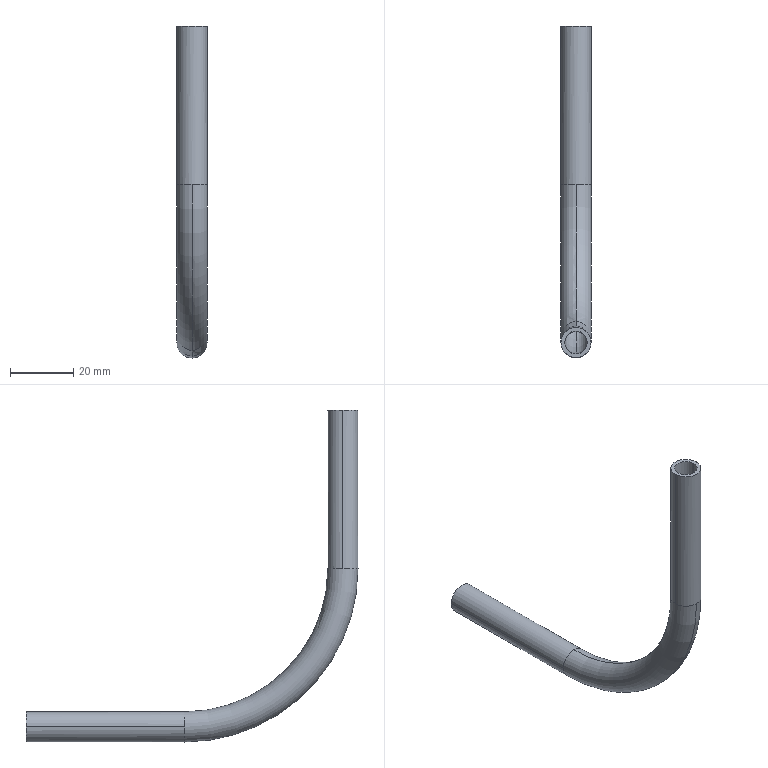Part | STEP file | TUBE-STS | 1 solid | 14 faces | box 9.52 x 104.76 x 104.76 mm | volume 5600 mm3 | cylinder 8 | torus 4 | plane 2 | commonest cylinder face diameters 7.12 x4 9.52 x4
STEP:
#1=CARTESIAN_POINT('',(0.,0.,0.));
#2=DIRECTION('',(0.,0.,1.));
#3=DIRECTION('',(1.,0.,0.));
#4=AXIS2_PLACEMENT_3D('',#1,#2,#3);
#5=CARTESIAN_POINT('',(-3.56,0.,-50.));
#6=VERTEX_POINT('',#5);
#7=CARTESIAN_POINT('',(0.,3.56,-50.));
#8=VERTEX_POINT('',#7);
#9=CARTESIAN_POINT('',(0.,0.,-50.));
#10=DIRECTION('',(0.,0.,-1.));
#11=DIRECTION('',(-1.,0.,0.));
#12=AXIS2_PLACEMENT_3D('',#9,#10,#11);
#13=CIRCLE('',#12,3.56);
#14=CARTESIAN_POINT('',(0.,50.,-50.));
#15=DIRECTION('',(1.,0.,0.));
#16=DIRECTION('',(0.,0.,-1.));
#17=AXIS2_PLACEMENT_3D('',#14,#15,#16);
#18=TOROIDAL_SURFACE('',#17,50.,3.56);
#19=CARTESIAN_POINT('',(4.712,4.712));
#20=DIRECTION('',(0.,-1.));
#21=VECTOR('',#20,1.);
#22=LINE('',#19,#21);
#23=(GEOMETRIC_REPRESENTATION_CONTEXT(2)PARAMETRIC_REPRESENTATION_CONTEXT()REPRESENTATION_CONTEXT('',''));
#24=DEFINITIONAL_REPRESENTATION('',(#22),#23);
#25=PCURVE('',#18,#24);
#26=CARTESIAN_POINT('',(0.,0.,0.));
#27=DIRECTION('',(0.,0.,-1.));
#28=DIRECTION('',(-1.,0.,0.));
#29=AXIS2_PLACEMENT_3D('',#26,#27,#28);
#30=CYLINDRICAL_SURFACE('',#29,3.56);
#31=CARTESIAN_POINT('',(0.,50.));
#32=DIRECTION('',(1.,0.));
#33=VECTOR('',#32,1.);
#34=LINE('',#31,#33);
#35=(GEOMETRIC_REPRESENTATION_CONTEXT(2)PARAMETRIC_REPRESENTATION_CONTEXT()REPRESENTATION_CONTEXT('',''));
#36=DEFINITIONAL_REPRESENTATION('',(#34),#35);
#37=PCURVE('',#30,#36);
#38=SURFACE_CURVE('',#13,(#25,#37),.PCURVE_S1.);
#39=EDGE_CURVE('',#6,#8,#38,.T.);
#40=ORIENTED_EDGE('',*,*,#39,.T.);
#41=CARTESIAN_POINT('',(0.,50.,-96.44));
#42=VERTEX_POINT('',#41);
#43=CARTESIAN_POINT('',(0.,50.,-50.));
#44=DIRECTION('',(1.,0.,0.));
#45=DIRECTION('',(0.,0.,-1.));
#46=AXIS2_PLACEMENT_3D('',#43,#44,#45);
#47=CIRCLE('',#46,46.44);
#48=CARTESIAN_POINT('',(0.,3.142));
#49=DIRECTION('',(1.,0.));
#50=VECTOR('',#49,1.);
#51=LINE('',#48,#50);
#52=(GEOMETRIC_REPRESENTATION_CONTEXT(2)PARAMETRIC_REPRESENTATION_CONTEXT()REPRESENTATION_CONTEXT('',''));
#53=DEFINITIONAL_REPRESENTATION('',(#51),#52);
#54=PCURVE('',#18,#53);
#55=CARTESIAN_POINT('',(0.,50.,-50.));
#56=DIRECTION('',(1.,0.,0.));
#57=DIRECTION('',(0.,0.,-1.));
#58=AXIS2_PLACEMENT_3D('',#55,#56,#57);
#59=TOROIDAL_SURFACE('',#58,50.,3.56);
#60=CARTESIAN_POINT('',(0.,3.142));
#61=DIRECTION('',(1.,0.));
#62=VECTOR('',#61,1.);
#63=LINE('',#60,#62);
#64=(GEOMETRIC_REPRESENTATION_CONTEXT(2)PARAMETRIC_REPRESENTATION_CONTEXT()REPRESENTATION_CONTEXT('',''));
#65=DEFINITIONAL_REPRESENTATION('',(#63),#64);
#66=PCURVE('',#59,#65);
#67=SURFACE_CURVE('',#47,(#54,#66),.PCURVE_S1.);
#68=EDGE_CURVE('',#8,#42,#67,.T.);
#69=ORIENTED_EDGE('',*,*,#68,.T.);
#70=CARTESIAN_POINT('',(-3.56,50.,-100.));
#71=VERTEX_POINT('',#70);
#72=CARTESIAN_POINT('',(0.,50.,-100.));
#73=DIRECTION('',(0.,1.,0.));
#74=DIRECTION('',(-1.,0.,0.));
#75=AXIS2_PLACEMENT_3D('',#72,#73,#74);
#76=CIRCLE('',#75,3.56);
#77=CARTESIAN_POINT('',(6.283,4.712));
#78=DIRECTION('',(0.,-1.));
#79=VECTOR('',#78,1.);
#80=LINE('',#77,#79);
#81=(GEOMETRIC_REPRESENTATION_CONTEXT(2)PARAMETRIC_REPRESENTATION_CONTEXT()REPRESENTATION_CONTEXT('',''));
#82=DEFINITIONAL_REPRESENTATION('',(#80),#81);
#83=PCURVE('',#18,#82);
#84=CARTESIAN_POINT('',(0.,50.,-100.));
#85=DIRECTION('',(0.,1.,0.));
#86=DIRECTION('',(-1.,0.,0.));
#87=AXIS2_PLACEMENT_3D('',#84,#85,#86);
#88=CYLINDRICAL_SURFACE('',#87,3.56);
#89=CARTESIAN_POINT('',(0.,0.));
#90=DIRECTION('',(1.,0.));
#91=VECTOR('',#90,1.);
#92=LINE('',#89,#91);
#93=(GEOMETRIC_REPRESENTATION_CONTEXT(2)PARAMETRIC_REPRESENTATION_CONTEXT()REPRESENTATION_CONTEXT('',''));
#94=DEFINITIONAL_REPRESENTATION('',(#92),#93);
#95=PCURVE('',#88,#94);
#96=SURFACE_CURVE('',#76,(#83,#95),.PCURVE_S1.);
#97=EDGE_CURVE('',#71,#42,#96,.T.);
#98=ORIENTED_EDGE('',*,*,#97,.F.);
#99=CARTESIAN_POINT('',(0.,50.,-103.56));
#100=VERTEX_POINT('',#99);
#101=CARTESIAN_POINT('',(0.,50.,-100.));
#102=DIRECTION('',(0.,1.,0.));
#103=DIRECTION('',(-1.,0.,0.));
#104=AXIS2_PLACEMENT_3D('',#101,#102,#103);
#105=CIRCLE('',#104,3.56);
#106=CARTESIAN_POINT('',(6.283,10.996));
#107=DIRECTION('',(0.,-1.));
#108=VECTOR('',#107,1.);
#109=LINE('',#106,#108);
#110=(GEOMETRIC_REPRESENTATION_CONTEXT(2)PARAMETRIC_REPRESENTATION_CONTEXT()REPRESENTATION_CONTEXT('',''));
#111=DEFINITIONAL_REPRESENTATION('',(#109),#110);
#112=PCURVE('',#18,#111);
#113=CARTESIAN_POINT('',(0.,50.,-100.));
#114=DIRECTION('',(0.,1.,0.));
#115=DIRECTION('',(-1.,0.,0.));
#116=AXIS2_PLACEMENT_3D('',#113,#114,#115);
#117=CYLINDRICAL_SURFACE('',#116,3.56);
#118=CARTESIAN_POINT('',(0.,0.));
#119=DIRECTION('',(1.,0.));
#120=VECTOR('',#119,1.);
#121=LINE('',#118,#120);
#122=(GEOMETRIC_REPRESENTATION_CONTEXT(2)PARAMETRIC_REPRESENTATION_CONTEXT()REPRESENTATION_CONTEXT('',''));
#123=DEFINITIONAL_REPRESENTATION('',(#121),#122);
#124=PCURVE('',#117,#123);
#125=SURFACE_CURVE('',#105,(#112,#124),.PCURVE_S1.);
#126=EDGE_CURVE('',#100,#71,#125,.T.);
#127=ORIENTED_EDGE('',*,*,#126,.F.);
#128=CARTESIAN_POINT('',(0.,-3.56,-50.));
#129=VERTEX_POINT('',#128);
#130=CARTESIAN_POINT('',(0.,50.,-50.));
#131=DIRECTION('',(1.,0.,0.));
#132=DIRECTION('',(0.,0.,-1.));
#133=AXIS2_PLACEMENT_3D('',#130,#131,#132);
#134=CIRCLE('',#133,53.56);
#135=CARTESIAN_POINT('',(0.,6.283));
#136=DIRECTION('',(1.,0.));
#137=VECTOR('',#136,1.);
#138=LINE('',#135,#137);
#139=(GEOMETRIC_REPRESENTATION_CONTEXT(2)PARAMETRIC_REPRESENTATION_CONTEXT()REPRESENTATION_CONTEXT('',''));
#140=DEFINITIONAL_REPRESENTATION('',(#138),#139);
#141=PCURVE('',#18,#140);
#142=CARTESIAN_POINT('',(0.,0.));
#143=DIRECTION('',(1.,0.));
#144=VECTOR('',#143,1.);
#145=LINE('',#142,#144);
#146=(GEOMETRIC_REPRESENTATION_CONTEXT(2)PARAMETRIC_REPRESENTATION_CONTEXT()REPRESENTATION_CONTEXT('',''));
#147=DEFINITIONAL_REPRESENTATION('',(#145),#146);
#148=PCURVE('',#59,#147);
#149=SURFACE_CURVE('',#134,(#141,#148),.PCURVE_S1.);
#150=EDGE_CURVE('',#129,#100,#149,.T.);
#151=ORIENTED_EDGE('',*,*,#150,.F.);
#152=CARTESIAN_POINT('',(0.,0.,-50.));
#153=DIRECTION('',(0.,0.,-1.));
#154=DIRECTION('',(-1.,0.,0.));
#155=AXIS2_PLACEMENT_3D('',#152,#153,#154);
#156=CIRCLE('',#155,3.56);
#157=CARTESIAN_POINT('',(4.712,10.996));
#158=DIRECTION('',(0.,-1.));
#159=VECTOR('',#158,1.);
#160=LINE('',#157,#159);
#161=(GEOMETRIC_REPRESENTATION_CONTEXT(2)PARAMETRIC_REPRESENTATION_CONTEXT()REPRESENTATION_CONTEXT('',''));
#162=DEFINITIONAL_REPRESENTATION('',(#160),#161);
#163=PCURVE('',#18,#162);
#164=CARTESIAN_POINT('',(0.,0.,0.));
#165=DIRECTION('',(0.,0.,-1.));
#166=DIRECTION('',(-1.,0.,0.));
#167=AXIS2_PLACEMENT_3D('',#164,#165,#166);
#168=CYLINDRICAL_SURFACE('',#167,3.56);
#169=CARTESIAN_POINT('',(0.,50.));
#170=DIRECTION('',(1.,0.));
#171=VECTOR('',#170,1.);
#172=LINE('',#169,#171);
#173=(GEOMETRIC_REPRESENTATION_CONTEXT(2)PARAMETRIC_REPRESENTATION_CONTEXT()REPRESENTATION_CONTEXT('',''));
#174=DEFINITIONAL_REPRESENTATION('',(#172),#173);
#175=PCURVE('',#168,#174);
#176=SURFACE_CURVE('',#156,(#163,#175),.PCURVE_S1.);
#177=EDGE_CURVE('',#129,#6,#176,.T.);
#178=ORIENTED_EDGE('',*,*,#177,.T.);
#179=EDGE_LOOP('',(#40,#69,#98,#127,#151,#178));
#180=FACE_BOUND('',#179,.F.);
#181=ADVANCED_FACE('',(#180),#18,.F.);
#182=CARTESIAN_POINT('',(4.76,0.,-50.));
#183=VERTEX_POINT('',#182);
#184=CARTESIAN_POINT('',(0.,-4.76,-50.));
#185=VERTEX_POINT('',#184);
#186=CARTESIAN_POINT('',(0.,0.,-50.));
#187=DIRECTION('',(0.,0.,-1.));
#188=DIRECTION('',(1.,0.,0.));
#189=AXIS2_PLACEMENT_3D('',#186,#187,#188);
#190=CIRCLE('',#189,4.76);
#191=CARTESIAN_POINT('',(0.,50.,-50.));
#192=DIRECTION('',(1.,0.,0.));
#193=DIRECTION('',(0.,0.,-1.));
#194=AXIS2_PLACEMENT_3D('',#191,#192,#193);
#195=TOROIDAL_SURFACE('',#194,50.,4.76);
#196=CARTESIAN_POINT('',(4.712,1.571));
#197=DIRECTION('',(0.,-1.));
#198=VECTOR('',#197,1.);
#199=LINE('',#196,#198);
#200=(GEOMETRIC_REPRESENTATION_CONTEXT(2)PARAMETRIC_REPRESENTATION_CONTEXT()REPRESENTATION_CONTEXT('',''));
#201=DEFINITIONAL_REPRESENTATION('',(#199),#200);
#202=PCURVE('',#195,#201);
#203=CARTESIAN_POINT('',(0.,0.,0.));
#204=DIRECTION('',(0.,0.,-1.));
#205=DIRECTION('',(1.,0.,0.));
#206=AXIS2_PLACEMENT_3D('',#203,#204,#205);
#207=CYLINDRICAL_SURFACE('',#206,4.76);
#208=CARTESIAN_POINT('',(0.,50.));
#209=DIRECTION('',(1.,0.));
#210=VECTOR('',#209,1.);
#211=LINE('',#208,#210);
#212=(GEOMETRIC_REPRESENTATION_CONTEXT(2)PARAMETRIC_REPRESENTATION_CONTEXT()REPRESENTATION_CONTEXT('',''));
#213=DEFINITIONAL_REPRESENTATION('',(#211),#212);
#214=PCURVE('',#207,#213);
#215=SURFACE_CURVE('',#190,(#202,#214),.PCURVE_S1.);
#216=EDGE_CURVE('',#183,#185,#215,.T.);
#217=ORIENTED_EDGE('',*,*,#216,.T.);
#218=CARTESIAN_POINT('',(0.,50.,-104.76));
#219=VERTEX_POINT('',#218);
#220=CARTESIAN_POINT('',(0.,50.,-50.));
#221=DIRECTION('',(1.,0.,0.));
#222=DIRECTION('',(0.,0.,-1.));
#223=AXIS2_PLACEMENT_3D('',#220,#221,#222);
#224=CIRCLE('',#223,54.76);
#225=CARTESIAN_POINT('',(0.,0.));
#226=DIRECTION('',(1.,0.));
#227=VECTOR('',#226,1.);
#228=LINE('',#225,#227);
#229=(GEOMETRIC_REPRESENTATION_CONTEXT(2)PARAMETRIC_REPRESENTATION_CONTEXT()REPRESENTATION_CONTEXT('',''));
#230=DEFINITIONAL_REPRESENTATION('',(#228),#229);
#231=PCURVE('',#195,#230);
#232=CARTESIAN_POINT('',(0.,50.,-50.));
#233=DIRECTION('',(1.,0.,0.));
#234=DIRECTION('',(0.,0.,-1.));
#235=AXIS2_PLACEMENT_3D('',#232,#233,#234);
#236=TOROIDAL_SURFACE('',#235,50.,4.76);
#237=CARTESIAN_POINT('',(0.,6.283));
#238=DIRECTION('',(1.,0.));
#239=VECTOR('',#238,1.);
#240=LINE('',#237,#239);
#241=(GEOMETRIC_REPRESENTATION_CONTEXT(2)PARAMETRIC_REPRESENTATION_CONTEXT()REPRESENTATION_CONTEXT('',''));
#242=DEFINITIONAL_REPRESENTATION('',(#240),#241);
#243=PCURVE('',#236,#242);
#244=SURFACE_CURVE('',#224,(#231,#243),.PCURVE_S1.);
#245=EDGE_CURVE('',#185,#219,#244,.T.);
#246=ORIENTED_EDGE('',*,*,#245,.T.);
#247=CARTESIAN_POINT('',(4.76,50.,-100.));
#248=VERTEX_POINT('',#247);
#249=CARTESIAN_POINT('',(0.,50.,-100.));
#250=DIRECTION('',(0.,1.,0.));
#251=DIRECTION('',(1.,0.,0.));
#252=AXIS2_PLACEMENT_3D('',#249,#250,#251);
#253=CIRCLE('',#252,4.76);
#254=CARTESIAN_POINT('',(6.283,1.571));
#255=DIRECTION('',(0.,-1.));
#256=VECTOR('',#255,1.);
#257=LINE('',#254,#256);
#258=(GEOMETRIC_REPRESENTATION_CONTEXT(2)PARAMETRIC_REPRESENTATION_CONTEXT()REPRESENTATION_CONTEXT('',''));
#259=DEFINITIONAL_REPRESENTATION('',(#257),#258);
#260=PCURVE('',#195,#259);
#261=CARTESIAN_POINT('',(0.,50.,-100.));
#262=DIRECTION('',(0.,1.,0.));
#263=DIRECTION('',(1.,0.,0.));
#264=AXIS2_PLACEMENT_3D('',#261,#262,#263);
#265=CYLINDRICAL_SURFACE('',#264,4.76);
#266=CARTESIAN_POINT('',(0.,0.));
#267=DIRECTION('',(1.,0.));
#268=VECTOR('',#267,1.);
#269=LINE('',#266,#268);
#270=(GEOMETRIC_REPRESENTATION_CONTEXT(2)PARAMETRIC_REPRESENTATION_CONTEXT()REPRESENTATION_CONTEXT('',''));
#271=DEFINITIONAL_REPRESENTATION('',(#269),#270);
#272=PCURVE('',#265,#271);
#273=SURFACE_CURVE('',#253,(#260,#272),.PCURVE_S1.);
#274=EDGE_CURVE('',#248,#219,#273,.T.);
#275=ORIENTED_EDGE('',*,*,#274,.F.);
#276=CARTESIAN_POINT('',(0.,50.,-95.24));
#277=VERTEX_POINT('',#276);
#278=CARTESIAN_POINT('',(0.,50.,-100.));
#279=DIRECTION('',(0.,1.,0.));
#280=DIRECTION('',(1.,0.,0.));
#281=AXIS2_PLACEMENT_3D('',#278,#279,#280);
#282=CIRCLE('',#281,4.76);
#283=CARTESIAN_POINT('',(6.283,7.854));
#284=DIRECTION('',(0.,-1.));
#285=VECTOR('',#284,1.);
#286=LINE('',#283,#285);
#287=(GEOMETRIC_REPRESENTATION_CONTEXT(2)PARAMETRIC_REPRESENTATION_CONTEXT()REPRESENTATION_CONTEXT('',''));
#288=DEFINITIONAL_REPRESENTATION('',(#286),#287);
#289=PCURVE('',#195,#288);
#290=CARTESIAN_POINT('',(0.,50.,-100.));
#291=DIRECTION('',(0.,1.,0.));
#292=DIRECTION('',(1.,0.,0.));
#293=AXIS2_PLACEMENT_3D('',#290,#291,#292);
#294=CYLINDRICAL_SURFACE('',#293,4.76);
#295=CARTESIAN_POINT('',(0.,0.));
#296=DIRECTION('',(1.,0.));
#297=VECTOR('',#296,1.);
#298=LINE('',#295,#297);
#299=(GEOMETRIC_REPRESENTATION_CONTEXT(2)PARAMETRIC_REPRESENTATION_CONTEXT()REPRESENTATION_CONTEXT('',''));
#300=DEFINITIONAL_REPRESENTATION('',(#298),#299);
#301=PCURVE('',#294,#300);
#302=SURFACE_CURVE('',#282,(#289,#301),.PCURVE_S1.);
#303=EDGE_CURVE('',#277,#248,#302,.T.);
#304=ORIENTED_EDGE('',*,*,#303,.F.);
#305=CARTESIAN_POINT('',(0.,4.76,-50.));
#306=VERTEX_POINT('',#305);
#307=CARTESIAN_POINT('',(0.,50.,-50.));
#308=DIRECTION('',(1.,0.,0.));
#309=DIRECTION('',(0.,0.,-1.));
#310=AXIS2_PLACEMENT_3D('',#307,#308,#309);
#311=CIRCLE('',#310,45.24);
#312=CARTESIAN_POINT('',(0.,3.142));
#313=DIRECTION('',(1.,0.));
#314=VECTOR('',#313,1.);
#315=LINE('',#312,#314);
#316=(GEOMETRIC_REPRESENTATION_CONTEXT(2)PARAMETRIC_REPRESENTATION_CONTEXT()REPRESENTATION_CONTEXT('',''));
#317=DEFINITIONAL_REPRESENTATION('',(#315),#316);
#318=PCURVE('',#195,#317);
#319=CARTESIAN_POINT('',(0.,3.142));
#320=DIRECTION('',(1.,0.));
#321=VECTOR('',#320,1.);
#322=LINE('',#319,#321);
#323=(GEOMETRIC_REPRESENTATION_CONTEXT(2)PARAMETRIC_REPRESENTATION_CONTEXT()REPRESENTATION_CONTEXT('',''));
#324=DEFINITIONAL_REPRESENTATION('',(#322),#323);
#325=PCURVE('',#236,#324);
#326=SURFACE_CURVE('',#311,(#318,#325),.PCURVE_S1.);
#327=EDGE_CURVE('',#306,#277,#326,.T.);
#328=ORIENTED_EDGE('',*,*,#327,.F.);
#329=CARTESIAN_POINT('',(0.,0.,-50.));
#330=DIRECTION('',(0.,0.,-1.));
#331=DIRECTION('',(1.,0.,0.));
#332=AXIS2_PLACEMENT_3D('',#329,#330,#331);
#333=CIRCLE('',#332,4.76);
#334=CARTESIAN_POINT('',(4.712,7.854));
#335=DIRECTION('',(0.,-1.));
#336=VECTOR('',#335,1.);
#337=LINE('',#334,#336);
#338=(GEOMETRIC_REPRESENTATION_CONTEXT(2)PARAMETRIC_REPRESENTATION_CONTEXT()REPRESENTATION_CONTEXT('',''));
#339=DEFINITIONAL_REPRESENTATION('',(#337),#338);
#340=PCURVE('',#195,#339);
#341=CARTESIAN_POINT('',(0.,0.,0.));
#342=DIRECTION('',(0.,0.,-1.));
#343=DIRECTION('',(1.,0.,0.));
#344=AXIS2_PLACEMENT_3D('',#341,#342,#343);
#345=CYLINDRICAL_SURFACE('',#344,4.76);
#346=CARTESIAN_POINT('',(0.,50.));
#347=DIRECTION('',(1.,0.));
#348=VECTOR('',#347,1.);
#349=LINE('',#346,#348);
#350=(GEOMETRIC_REPRESENTATION_CONTEXT(2)PARAMETRIC_REPRESENTATION_CONTEXT()REPRESENTATION_CONTEXT('',''));
#351=DEFINITIONAL_REPRESENTATION('',(#349),#350);
#352=PCURVE('',#345,#351);
#353=SURFACE_CURVE('',#333,(#340,#352),.PCURVE_S1.);
#354=EDGE_CURVE('',#306,#183,#353,.T.);
#355=ORIENTED_EDGE('',*,*,#354,.T.);
#356=EDGE_LOOP('',(#217,#246,#275,#304,#328,#355));
#357=FACE_BOUND('',#356,.T.);
#358=ADVANCED_FACE('',(#357),#195,.T.);
#359=ORIENTED_EDGE('',*,*,#126,.T.);
#360=CARTESIAN_POINT('',(-3.56,100.,-100.));
#361=VERTEX_POINT('',#360);
#362=CARTESIAN_POINT('',(-3.56,50.,-100.));
#363=DIRECTION('',(0.,1.,0.));
#364=VECTOR('',#363,1.);
#365=LINE('',#362,#364);
#366=CARTESIAN_POINT('',(6.283,0.));
#367=DIRECTION('',(0.,1.));
#368=VECTOR('',#367,1.);
#369=LINE('',#366,#368);
#370=(GEOMETRIC_REPRESENTATION_CONTEXT(2)PARAMETRIC_REPRESENTATION_CONTEXT()REPRESENTATION_CONTEXT('',''));
#371=DEFINITIONAL_REPRESENTATION('',(#369),#370);
#372=PCURVE('',#117,#371);
#373=CARTESIAN_POINT('',(0.,0.));
#374=DIRECTION('',(0.,1.));
#375=VECTOR('',#374,1.);
#376=LINE('',#373,#375);
#377=(GEOMETRIC_REPRESENTATION_CONTEXT(2)PARAMETRIC_REPRESENTATION_CONTEXT()REPRESENTATION_CONTEXT('',''));
#378=DEFINITIONAL_REPRESENTATION('',(#376),#377);
#379=PCURVE('',#88,#378);
#380=SURFACE_CURVE('',#365,(#372,#379),.PCURVE_S1.);
#381=EDGE_CURVE('',#71,#361,#380,.T.);
#382=ORIENTED_EDGE('',*,*,#381,.T.);
#383=CARTESIAN_POINT('',(3.56,100.,-100.));
#384=VERTEX_POINT('',#383);
#385=CARTESIAN_POINT('',(0.,100.,-100.));
#386=DIRECTION('',(0.,-1.,0.));
#387=DIRECTION('',(-1.,0.,0.));
#388=AXIS2_PLACEMENT_3D('',#385,#386,#387);
#389=CIRCLE('',#388,3.56);
#390=CARTESIAN_POINT('',(6.283,50.));
#391=DIRECTION('',(-1.,0.));
#392=VECTOR('',#391,1.);
#393=LINE('',#390,#392);
#394=(GEOMETRIC_REPRESENTATION_CONTEXT(2)PARAMETRIC_REPRESENTATION_CONTEXT()REPRESENTATION_CONTEXT('',''));
#395=DEFINITIONAL_REPRESENTATION('',(#393),#394);
#396=PCURVE('',#117,#395);
#397=CARTESIAN_POINT('',(0.,100.,-100.));
#398=DIRECTION('',(0.,-1.,0.));
#399=DIRECTION('',(-1.,0.,0.));
#400=AXIS2_PLACEMENT_3D('',#397,#398,#399);
#401=PLANE('',#400);
#402=CARTESIAN_POINT('',(0.,0.));
#403=DIRECTION('',(1.,0.));
#404=AXIS2_PLACEMENT_2D('',#402,#403);
#405=CIRCLE('',#404,3.56);
#406=(GEOMETRIC_REPRESENTATION_CONTEXT(2)PARAMETRIC_REPRESENTATION_CONTEXT()REPRESENTATION_CONTEXT('',''));
#407=DEFINITIONAL_REPRESENTATION('',(#405),#406);
#408=PCURVE('',#401,#407);
#409=SURFACE_CURVE('',#389,(#396,#408),.PCURVE_S1.);
#410=EDGE_CURVE('',#361,#384,#409,.T.);
#411=ORIENTED_EDGE('',*,*,#410,.T.);
#412=CARTESIAN_POINT('',(3.56,50.,-100.));
#413=VERTEX_POINT('',#412);
#414=CARTESIAN_POINT('',(3.56,50.,-100.));
#415=DIRECTION('',(0.,1.,0.));
#416=VECTOR('',#415,1.);
#417=LINE('',#414,#416);
#418=CARTESIAN_POINT('',(3.142,0.));
#419=DIRECTION('',(0.,1.));
#420=VECTOR('',#419,1.);
#421=LINE('',#418,#420);
#422=(GEOMETRIC_REPRESENTATION_CONTEXT(2)PARAMETRIC_REPRESENTATION_CONTEXT()REPRESENTATION_CONTEXT('',''));
#423=DEFINITIONAL_REPRESENTATION('',(#421),#422);
#424=PCURVE('',#117,#423);
#425=CARTESIAN_POINT('',(3.142,0.));
#426=DIRECTION('',(0.,1.));
#427=VECTOR('',#426,1.);
#428=LINE('',#425,#427);
#429=(GEOMETRIC_REPRESENTATION_CONTEXT(2)PARAMETRIC_REPRESENTATION_CONTEXT()REPRESENTATION_CONTEXT('',''));
#430=DEFINITIONAL_REPRESENTATION('',(#428),#429);
#431=PCURVE('',#88,#430);
#432=SURFACE_CURVE('',#417,(#424,#431),.PCURVE_S1.);
#433=EDGE_CURVE('',#413,#384,#432,.T.);
#434=ORIENTED_EDGE('',*,*,#433,.F.);
#435=CARTESIAN_POINT('',(0.,50.,-100.));
#436=DIRECTION('',(0.,1.,0.));
#437=DIRECTION('',(-1.,0.,0.));
#438=AXIS2_PLACEMENT_3D('',#435,#436,#437);
#439=CIRCLE('',#438,3.56);
#440=CARTESIAN_POINT('',(0.,0.));
#441=DIRECTION('',(1.,0.));
#442=VECTOR('',#441,1.);
#443=LINE('',#440,#442);
#444=(GEOMETRIC_REPRESENTATION_CONTEXT(2)PARAMETRIC_REPRESENTATION_CONTEXT()REPRESENTATION_CONTEXT('',''));
#445=DEFINITIONAL_REPRESENTATION('',(#443),#444);
#446=PCURVE('',#117,#445);
#447=CARTESIAN_POINT('',(6.283,4.712));
#448=DIRECTION('',(0.,-1.));
#449=VECTOR('',#448,1.);
#450=LINE('',#447,#449);
#451=(GEOMETRIC_REPRESENTATION_CONTEXT(2)PARAMETRIC_REPRESENTATION_CONTEXT()REPRESENTATION_CONTEXT('',''));
#452=DEFINITIONAL_REPRESENTATION('',(#450),#451);
#453=PCURVE('',#59,#452);
#454=SURFACE_CURVE('',#439,(#446,#453),.PCURVE_S1.);
#455=EDGE_CURVE('',#413,#100,#454,.T.);
#456=ORIENTED_EDGE('',*,*,#455,.T.);
#457=EDGE_LOOP('',(#359,#382,#411,#434,#456));
#458=FACE_BOUND('',#457,.F.);
#459=ADVANCED_FACE('',(#458),#117,.F.);
#460=CARTESIAN_POINT('',(-3.56,0.,0.));
#461=VERTEX_POINT('',#460);
#462=CARTESIAN_POINT('',(-3.56,0.,0.));
#463=DIRECTION('',(0.,0.,-1.));
#464=VECTOR('',#463,1.);
#465=LINE('',#462,#464);
#466=CARTESIAN_POINT('',(6.283,0.));
#467=DIRECTION('',(0.,1.));
#468=VECTOR('',#467,1.);
#469=LINE('',#466,#468);
#470=(GEOMETRIC_REPRESENTATION_CONTEXT(2)PARAMETRIC_REPRESENTATION_CONTEXT()REPRESENTATION_CONTEXT('',''));
#471=DEFINITIONAL_REPRESENTATION('',(#469),#470);
#472=PCURVE('',#168,#471);
#473=CARTESIAN_POINT('',(0.,0.));
#474=DIRECTION('',(0.,1.));
#475=VECTOR('',#474,1.);
#476=LINE('',#473,#475);
#477=(GEOMETRIC_REPRESENTATION_CONTEXT(2)PARAMETRIC_REPRESENTATION_CONTEXT()REPRESENTATION_CONTEXT('',''));
#478=DEFINITIONAL_REPRESENTATION('',(#476),#477);
#479=PCURVE('',#30,#478);
#480=SURFACE_CURVE('',#465,(#472,#479),.PCURVE_S1.);
#481=EDGE_CURVE('',#461,#6,#480,.T.);
#482=ORIENTED_EDGE('',*,*,#481,.T.);
#483=ORIENTED_EDGE('',*,*,#177,.F.);
#484=CARTESIAN_POINT('',(3.56,0.,-50.));
#485=VERTEX_POINT('',#484);
#486=CARTESIAN_POINT('',(0.,0.,-50.));
#487=DIRECTION('',(0.,0.,-1.));
#488=DIRECTION('',(-1.,0.,0.));
#489=AXIS2_PLACEMENT_3D('',#486,#487,#488);
#490=CIRCLE('',#489,3.56);
#491=CARTESIAN_POINT('',(0.,50.));
#492=DIRECTION('',(1.,0.));
#493=VECTOR('',#492,1.);
#494=LINE('',#491,#493);
#495=(GEOMETRIC_REPRESENTATION_CONTEXT(2)PARAMETRIC_REPRESENTATION_CONTEXT()REPRESENTATION_CONTEXT('',''));
#496=DEFINITIONAL_REPRESENTATION('',(#494),#495);
#497=PCURVE('',#168,#496);
#498=CARTESIAN_POINT('',(4.712,4.712));
#499=DIRECTION('',(0.,-1.));
#500=VECTOR('',#499,1.);
#501=LINE('',#498,#500);
#502=(GEOMETRIC_REPRESENTATION_CONTEXT(2)PARAMETRIC_REPRESENTATION_CONTEXT()REPRESENTATION_CONTEXT('',''));
#503=DEFINITIONAL_REPRESENTATION('',(#501),#502);
#504=PCURVE('',#59,#503);
#505=SURFACE_CURVE('',#490,(#497,#504),.PCURVE_S1.);
#506=EDGE_CURVE('',#485,#129,#505,.T.);
#507=ORIENTED_EDGE('',*,*,#506,.F.);
#508=CARTESIAN_POINT('',(3.56,0.,0.));
#509=VERTEX_POINT('',#508);
#510=CARTESIAN_POINT('',(3.56,0.,0.));
#511=DIRECTION('',(0.,0.,-1.));
#512=VECTOR('',#511,1.);
#513=LINE('',#510,#512);
#514=CARTESIAN_POINT('',(3.142,0.));
#515=DIRECTION('',(0.,1.));
#516=VECTOR('',#515,1.);
#517=LINE('',#514,#516);
#518=(GEOMETRIC_REPRESENTATION_CONTEXT(2)PARAMETRIC_REPRESENTATION_CONTEXT()REPRESENTATION_CONTEXT('',''));
#519=DEFINITIONAL_REPRESENTATION('',(#517),#518);
#520=PCURVE('',#168,#519);
#521=CARTESIAN_POINT('',(3.142,0.));
#522=DIRECTION('',(0.,1.));
#523=VECTOR('',#522,1.);
#524=LINE('',#521,#523);
#525=(GEOMETRIC_REPRESENTATION_CONTEXT(2)PARAMETRIC_REPRESENTATION_CONTEXT()REPRESENTATION_CONTEXT('',''));
#526=DEFINITIONAL_REPRESENTATION('',(#524),#525);
#527=PCURVE('',#30,#526);
#528=SURFACE_CURVE('',#513,(#520,#527),.PCURVE_S1.);
#529=EDGE_CURVE('',#509,#485,#528,.T.);
#530=ORIENTED_EDGE('',*,*,#529,.F.);
#531=CARTESIAN_POINT('',(0.,0.,0.));
#532=DIRECTION('',(0.,0.,-1.));
#533=DIRECTION('',(-1.,0.,0.));
#534=AXIS2_PLACEMENT_3D('',#531,#532,#533);
#535=CIRCLE('',#534,3.56);
#536=CARTESIAN_POINT('',(0.,0.));
#537=DIRECTION('',(1.,0.));
#538=VECTOR('',#537,1.);
#539=LINE('',#536,#538);
#540=(GEOMETRIC_REPRESENTATION_CONTEXT(2)PARAMETRIC_REPRESENTATION_CONTEXT()REPRESENTATION_CONTEXT('',''));
#541=DEFINITIONAL_REPRESENTATION('',(#539),#540);
#542=PCURVE('',#168,#541);
#543=CARTESIAN_POINT('',(0.,0.,0.));
#544=DIRECTION('',(0.,0.,1.));
#545=DIRECTION('',(1.,0.,0.));
#546=AXIS2_PLACEMENT_3D('',#543,#544,#545);
#547=PLANE('',#546);
#548=CARTESIAN_POINT('',(-3.56,0.));
#549=CARTESIAN_POINT('',(-3.56,6.166));
#550=CARTESIAN_POINT('',(1.78,3.083));
#551=CARTESIAN_POINT('',(7.12,0.));
#552=CARTESIAN_POINT('',(1.78,-3.083));
#553=CARTESIAN_POINT('',(-3.56,-6.166));
#554=CARTESIAN_POINT('',(-3.56,0.));
#555=(BOUNDED_CURVE()B_SPLINE_CURVE(2,(#548,#549,#550,#551,#552,#553,#554),.UNSPECIFIED.,.T.,.F.)B_SPLINE_CURVE_WITH_KNOTS((1,2,2,2,2,1),(-2.094,0.,2.094,4.189,6.283,8.378),.UNSPECIFIED.)CURVE()GEOMETRIC_REPRESENTATION_ITEM()RATIONAL_B_SPLINE_CURVE((1.,0.5,1.,0.5,1.,0.5,1.))REPRESENTATION_ITEM(''));
#556=(GEOMETRIC_REPRESENTATION_CONTEXT(2)PARAMETRIC_REPRESENTATION_CONTEXT()REPRESENTATION_CONTEXT('',''));
#557=DEFINITIONAL_REPRESENTATION('',(#555),#556);
#558=PCURVE('',#547,#557);
#559=SURFACE_CURVE('',#535,(#542,#558),.PCURVE_S1.);
#560=EDGE_CURVE('',#509,#461,#559,.T.);
#561=ORIENTED_EDGE('',*,*,#560,.T.);
#562=EDGE_LOOP('',(#482,#483,#507,#530,#561));
#563=FACE_BOUND('',#562,.F.);
#564=ADVANCED_FACE('',(#563),#168,.F.);
#565=ORIENTED_EDGE('',*,*,#274,.T.);
#566=CARTESIAN_POINT('',(-4.76,50.,-100.));
#567=VERTEX_POINT('',#566);
#568=CARTESIAN_POINT('',(0.,50.,-100.));
#569=DIRECTION('',(0.,1.,0.));
#570=DIRECTION('',(1.,0.,0.));
#571=AXIS2_PLACEMENT_3D('',#568,#569,#570);
#572=CIRCLE('',#571,4.76);
#573=CARTESIAN_POINT('',(0.,0.));
#574=DIRECTION('',(1.,0.));
#575=VECTOR('',#574,1.);
#576=LINE('',#573,#575);
#577=(GEOMETRIC_REPRESENTATION_CONTEXT(2)PARAMETRIC_REPRESENTATION_CONTEXT()REPRESENTATION_CONTEXT('',''));
#578=DEFINITIONAL_REPRESENTATION('',(#576),#577);
#579=PCURVE('',#265,#578);
#580=CARTESIAN_POINT('',(6.283,7.854));
#581=DIRECTION('',(0.,-1.));
#582=VECTOR('',#581,1.);
#583=LINE('',#580,#582);
#584=(GEOMETRIC_REPRESENTATION_CONTEXT(2)PARAMETRIC_REPRESENTATION_CONTEXT()REPRESENTATION_CONTEXT('',''));
#585=DEFINITIONAL_REPRESENTATION('',(#583),#584);
#586=PCURVE('',#236,#585);
#587=SURFACE_CURVE('',#572,(#579,#586),.PCURVE_S1.);
#588=EDGE_CURVE('',#219,#567,#587,.T.);
#589=ORIENTED_EDGE('',*,*,#588,.T.);
#590=CARTESIAN_POINT('',(-4.76,100.,-100.));
#591=VERTEX_POINT('',#590);
#592=CARTESIAN_POINT('',(-4.76,50.,-100.));
#593=DIRECTION('',(0.,1.,0.));
#594=VECTOR('',#593,1.);
#595=LINE('',#592,#594);
#596=CARTESIAN_POINT('',(3.142,0.));
#597=DIRECTION('',(0.,1.));
#598=VECTOR('',#597,1.);
#599=LINE('',#596,#598);
#600=(GEOMETRIC_REPRESENTATION_CONTEXT(2)PARAMETRIC_REPRESENTATION_CONTEXT()REPRESENTATION_CONTEXT('',''));
#601=DEFINITIONAL_REPRESENTATION('',(#599),#600);
#602=PCURVE('',#265,#601);
#603=CARTESIAN_POINT('',(3.142,0.));
#604=DIRECTION('',(0.,1.));
#605=VECTOR('',#604,1.);
#606=LINE('',#603,#605);
#607=(GEOMETRIC_REPRESENTATION_CONTEXT(2)PARAMETRIC_REPRESENTATION_CONTEXT()REPRESENTATION_CONTEXT('',''));
#608=DEFINITIONAL_REPRESENTATION('',(#606),#607);
#609=PCURVE('',#294,#608);
#610=SURFACE_CURVE('',#595,(#602,#609),.PCURVE_S1.);
#611=EDGE_CURVE('',#567,#591,#610,.T.);
#612=ORIENTED_EDGE('',*,*,#611,.T.);
#613=CARTESIAN_POINT('',(4.76,100.,-100.));
#614=VERTEX_POINT('',#613);
#615=CARTESIAN_POINT('',(0.,100.,-100.));
#616=DIRECTION('',(0.,1.,0.));
#617=DIRECTION('',(1.,0.,0.));
#618=AXIS2_PLACEMENT_3D('',#615,#616,#617);
#619=CIRCLE('',#618,4.76);
#620=CARTESIAN_POINT('',(0.,50.));
#621=DIRECTION('',(1.,0.));
#622=VECTOR('',#621,1.);
#623=LINE('',#620,#622);
#624=(GEOMETRIC_REPRESENTATION_CONTEXT(2)PARAMETRIC_REPRESENTATION_CONTEXT()REPRESENTATION_CONTEXT('',''));
#625=DEFINITIONAL_REPRESENTATION('',(#623),#624);
#626=PCURVE('',#265,#625);
#627=CARTESIAN_POINT('',(-4.76,0.));
#628=CARTESIAN_POINT('',(-4.76,8.245));
#629=CARTESIAN_POINT('',(2.38,4.122));
#630=CARTESIAN_POINT('',(9.52,0.));
#631=CARTESIAN_POINT('',(2.38,-4.122));
#632=CARTESIAN_POINT('',(-4.76,-8.245));
#633=CARTESIAN_POINT('',(-4.76,0.));
#634=(BOUNDED_CURVE()B_SPLINE_CURVE(2,(#627,#628,#629,#630,#631,#632,#633),.UNSPECIFIED.,.T.,.F.)B_SPLINE_CURVE_WITH_KNOTS((1,2,2,2,2,1),(-2.094,0.,2.094,4.189,6.283,8.378),.UNSPECIFIED.)CURVE()GEOMETRIC_REPRESENTATION_ITEM()RATIONAL_B_SPLINE_CURVE((1.,0.5,1.,0.5,1.,0.5,1.))REPRESENTATION_ITEM(''));
#635=(GEOMETRIC_REPRESENTATION_CONTEXT(2)PARAMETRIC_REPRESENTATION_CONTEXT()REPRESENTATION_CONTEXT('',''));
#636=DEFINITIONAL_REPRESENTATION('',(#634),#635);
#637=PCURVE('',#401,#636);
#638=SURFACE_CURVE('',#619,(#626,#637),.PCURVE_S1.);
#639=EDGE_CURVE('',#614,#591,#638,.T.);
#640=ORIENTED_EDGE('',*,*,#639,.F.);
#641=CARTESIAN_POINT('',(4.76,50.,-100.));
#642=DIRECTION('',(0.,1.,0.));
#643=VECTOR('',#642,1.);
#644=LINE('',#641,#643);
#645=CARTESIAN_POINT('',(0.,0.));
#646=DIRECTION('',(0.,1.));
#647=VECTOR('',#646,1.);
#648=LINE('',#645,#647);
#649=(GEOMETRIC_REPRESENTATION_CONTEXT(2)PARAMETRIC_REPRESENTATION_CONTEXT()REPRESENTATION_CONTEXT('',''));
#650=DEFINITIONAL_REPRESENTATION('',(#648),#649);
#651=PCURVE('',#265,#650);
#652=CARTESIAN_POINT('',(6.283,0.));
#653=DIRECTION('',(0.,1.));
#654=VECTOR('',#653,1.);
#655=LINE('',#652,#654);
#656=(GEOMETRIC_REPRESENTATION_CONTEXT(2)PARAMETRIC_REPRESENTATION_CONTEXT()REPRESENTATION_CONTEXT('',''));
#657=DEFINITIONAL_REPRESENTATION('',(#655),#656);
#658=PCURVE('',#294,#657);
#659=SURFACE_CURVE('',#644,(#651,#658),.PCURVE_S1.);
#660=EDGE_CURVE('',#248,#614,#659,.T.);
#661=ORIENTED_EDGE('',*,*,#660,.F.);
#662=EDGE_LOOP('',(#565,#589,#612,#640,#661));
#663=FACE_BOUND('',#662,.T.);
#664=ADVANCED_FACE('',(#663),#265,.T.);
#665=CARTESIAN_POINT('',(-4.76,0.,0.));
#666=VERTEX_POINT('',#665);
#667=CARTESIAN_POINT('',(4.76,0.,0.));
#668=VERTEX_POINT('',#667);
#669=CARTESIAN_POINT('',(0.,0.,0.));
#670=DIRECTION('',(0.,0.,1.));
#671=DIRECTION('',(1.,0.,0.));
#672=AXIS2_PLACEMENT_3D('',#669,#670,#671);
#673=CIRCLE('',#672,4.76);
#674=CARTESIAN_POINT('',(6.283,0.));
#675=DIRECTION('',(-1.,0.));
#676=VECTOR('',#675,1.);
#677=LINE('',#674,#676);
#678=(GEOMETRIC_REPRESENTATION_CONTEXT(2)PARAMETRIC_REPRESENTATION_CONTEXT()REPRESENTATION_CONTEXT('',''));
#679=DEFINITIONAL_REPRESENTATION('',(#677),#678);
#680=PCURVE('',#207,#679);
#681=CARTESIAN_POINT('',(0.,0.));
#682=DIRECTION('',(1.,0.));
#683=AXIS2_PLACEMENT_2D('',#681,#682);
#684=CIRCLE('',#683,4.76);
#685=(GEOMETRIC_REPRESENTATION_CONTEXT(2)PARAMETRIC_REPRESENTATION_CONTEXT()REPRESENTATION_CONTEXT('',''));
#686=DEFINITIONAL_REPRESENTATION('',(#684),#685);
#687=PCURVE('',#547,#686);
#688=SURFACE_CURVE('',#673,(#680,#687),.PCURVE_S1.);
#689=EDGE_CURVE('',#666,#668,#688,.T.);
#690=ORIENTED_EDGE('',*,*,#689,.F.);
#691=CARTESIAN_POINT('',(-4.76,0.,-50.));
#692=VERTEX_POINT('',#691);
#693=CARTESIAN_POINT('',(-4.76,0.,0.));
#694=DIRECTION('',(0.,0.,-1.));
#695=VECTOR('',#694,1.);
#696=LINE('',#693,#695);
#697=CARTESIAN_POINT('',(3.142,0.));
#698=DIRECTION('',(0.,1.));
#699=VECTOR('',#698,1.);
#700=LINE('',#697,#699);
#701=(GEOMETRIC_REPRESENTATION_CONTEXT(2)PARAMETRIC_REPRESENTATION_CONTEXT()REPRESENTATION_CONTEXT('',''));
#702=DEFINITIONAL_REPRESENTATION('',(#700),#701);
#703=PCURVE('',#207,#702);
#704=CARTESIAN_POINT('',(3.142,0.));
#705=DIRECTION('',(0.,1.));
#706=VECTOR('',#705,1.);
#707=LINE('',#704,#706);
#708=(GEOMETRIC_REPRESENTATION_CONTEXT(2)PARAMETRIC_REPRESENTATION_CONTEXT()REPRESENTATION_CONTEXT('',''));
#709=DEFINITIONAL_REPRESENTATION('',(#707),#708);
#710=PCURVE('',#345,#709);
#711=SURFACE_CURVE('',#696,(#703,#710),.PCURVE_S1.);
#712=EDGE_CURVE('',#666,#692,#711,.T.);
#713=ORIENTED_EDGE('',*,*,#712,.T.);
#714=CARTESIAN_POINT('',(0.,0.,-50.));
#715=DIRECTION('',(0.,0.,-1.));
#716=DIRECTION('',(1.,0.,0.));
#717=AXIS2_PLACEMENT_3D('',#714,#715,#716);
#718=CIRCLE('',#717,4.76);
#719=CARTESIAN_POINT('',(0.,50.));
#720=DIRECTION('',(1.,0.));
#721=VECTOR('',#720,1.);
#722=LINE('',#719,#721);
#723=(GEOMETRIC_REPRESENTATION_CONTEXT(2)PARAMETRIC_REPRESENTATION_CONTEXT()REPRESENTATION_CONTEXT('',''));
#724=DEFINITIONAL_REPRESENTATION('',(#722),#723);
#725=PCURVE('',#207,#724);
#726=CARTESIAN_POINT('',(4.712,7.854));
#727=DIRECTION('',(0.,-1.));
#728=VECTOR('',#727,1.);
#729=LINE('',#726,#728);
#730=(GEOMETRIC_REPRESENTATION_CONTEXT(2)PARAMETRIC_REPRESENTATION_CONTEXT()REPRESENTATION_CONTEXT('',''));
#731=DEFINITIONAL_REPRESENTATION('',(#729),#730);
#732=PCURVE('',#236,#731);
#733=SURFACE_CURVE('',#718,(#725,#732),.PCURVE_S1.);
#734=EDGE_CURVE('',#185,#692,#733,.T.);
#735=ORIENTED_EDGE('',*,*,#734,.F.);
#736=ORIENTED_EDGE('',*,*,#216,.F.);
#737=CARTESIAN_POINT('',(4.76,0.,0.));
#738=DIRECTION('',(0.,0.,-1.));
#739=VECTOR('',#738,1.);
#740=LINE('',#737,#739);
#741=CARTESIAN_POINT('',(0.,0.));
#742=DIRECTION('',(0.,1.));
#743=VECTOR('',#742,1.);
#744=LINE('',#741,#743);
#745=(GEOMETRIC_REPRESENTATION_CONTEXT(2)PARAMETRIC_REPRESENTATION_CONTEXT()REPRESENTATION_CONTEXT('',''));
#746=DEFINITIONAL_REPRESENTATION('',(#744),#745);
#747=PCURVE('',#207,#746);
#748=CARTESIAN_POINT('',(6.283,0.));
#749=DIRECTION('',(0.,1.));
#750=VECTOR('',#749,1.);
#751=LINE('',#748,#750);
#752=(GEOMETRIC_REPRESENTATION_CONTEXT(2)PARAMETRIC_REPRESENTATION_CONTEXT()REPRESENTATION_CONTEXT('',''));
#753=DEFINITIONAL_REPRESENTATION('',(#751),#752);
#754=PCURVE('',#345,#753);
#755=SURFACE_CURVE('',#740,(#747,#754),.PCURVE_S1.);
#756=EDGE_CURVE('',#668,#183,#755,.T.);
#757=ORIENTED_EDGE('',*,*,#756,.F.);
#758=EDGE_LOOP('',(#690,#713,#735,#736,#757));
#759=FACE_BOUND('',#758,.T.);
#760=ADVANCED_FACE('',(#759),#207,.T.);
#761=ORIENTED_EDGE('',*,*,#410,.T.);
#762=CARTESIAN_POINT('',(0.,100.,-100.));
#763=DIRECTION('',(0.,-1.,0.));
#764=DIRECTION('',(-1.,0.,0.));
#765=AXIS2_PLACEMENT_3D('',#762,#763,#764);
#766=CIRCLE('',#765,3.56);
#767=CARTESIAN_POINT('',(0.,0.));
#768=DIRECTION('',(1.,0.));
#769=AXIS2_PLACEMENT_2D('',#767,#768);
#770=CIRCLE('',#769,3.56);
#771=(GEOMETRIC_REPRESENTATION_CONTEXT(2)PARAMETRIC_REPRESENTATION_CONTEXT()REPRESENTATION_CONTEXT('',''));
#772=DEFINITIONAL_REPRESENTATION('',(#770),#771);
#773=PCURVE('',#401,#772);
#774=CARTESIAN_POINT('',(6.283,50.));
#775=DIRECTION('',(-1.,0.));
#776=VECTOR('',#775,1.);
#777=LINE('',#774,#776);
#778=(GEOMETRIC_REPRESENTATION_CONTEXT(2)PARAMETRIC_REPRESENTATION_CONTEXT()REPRESENTATION_CONTEXT('',''));
#779=DEFINITIONAL_REPRESENTATION('',(#777),#778);
#780=PCURVE('',#88,#779);
#781=SURFACE_CURVE('',#766,(#773,#780),.PCURVE_S1.);
#782=EDGE_CURVE('',#384,#361,#781,.T.);
#783=ORIENTED_EDGE('',*,*,#782,.T.);
#784=EDGE_LOOP('',(#761,#783));
#785=FACE_BOUND('',#784,.T.);
#786=ORIENTED_EDGE('',*,*,#639,.T.);
#787=CARTESIAN_POINT('',(0.,100.,-100.));
#788=DIRECTION('',(0.,1.,0.));
#789=DIRECTION('',(1.,0.,0.));
#790=AXIS2_PLACEMENT_3D('',#787,#788,#789);
#791=CIRCLE('',#790,4.76);
#792=CARTESIAN_POINT('',(-4.76,0.));
#793=CARTESIAN_POINT('',(-4.76,8.245));
#794=CARTESIAN_POINT('',(2.38,4.122));
#795=CARTESIAN_POINT('',(9.52,0.));
#796=CARTESIAN_POINT('',(2.38,-4.122));
#797=CARTESIAN_POINT('',(-4.76,-8.245));
#798=CARTESIAN_POINT('',(-4.76,0.));
#799=(BOUNDED_CURVE()B_SPLINE_CURVE(2,(#792,#793,#794,#795,#796,#797,#798),.UNSPECIFIED.,.T.,.F.)B_SPLINE_CURVE_WITH_KNOTS((1,2,2,2,2,1),(-2.094,0.,2.094,4.189,6.283,8.378),.UNSPECIFIED.)CURVE()GEOMETRIC_REPRESENTATION_ITEM()RATIONAL_B_SPLINE_CURVE((1.,0.5,1.,0.5,1.,0.5,1.))REPRESENTATION_ITEM(''));
#800=(GEOMETRIC_REPRESENTATION_CONTEXT(2)PARAMETRIC_REPRESENTATION_CONTEXT()REPRESENTATION_CONTEXT('',''));
#801=DEFINITIONAL_REPRESENTATION('',(#799),#800);
#802=PCURVE('',#401,#801);
#803=CARTESIAN_POINT('',(0.,50.));
#804=DIRECTION('',(1.,0.));
#805=VECTOR('',#804,1.);
#806=LINE('',#803,#805);
#807=(GEOMETRIC_REPRESENTATION_CONTEXT(2)PARAMETRIC_REPRESENTATION_CONTEXT()REPRESENTATION_CONTEXT('',''));
#808=DEFINITIONAL_REPRESENTATION('',(#806),#807);
#809=PCURVE('',#294,#808);
#810=SURFACE_CURVE('',#791,(#802,#809),.PCURVE_S1.);
#811=EDGE_CURVE('',#591,#614,#810,.T.);
#812=ORIENTED_EDGE('',*,*,#811,.T.);
#813=EDGE_LOOP('',(#786,#812));
#814=FACE_BOUND('',#813,.T.);
#815=ADVANCED_FACE('',(#785,#814),#401,.F.);
#816=CARTESIAN_POINT('',(0.,0.,0.));
#817=DIRECTION('',(0.,0.,-1.));
#818=DIRECTION('',(-1.,0.,0.));
#819=AXIS2_PLACEMENT_3D('',#816,#817,#818);
#820=CIRCLE('',#819,3.56);
#821=CARTESIAN_POINT('',(-3.56,0.));
#822=CARTESIAN_POINT('',(-3.56,6.166));
#823=CARTESIAN_POINT('',(1.78,3.083));
#824=CARTESIAN_POINT('',(7.12,0.));
#825=CARTESIAN_POINT('',(1.78,-3.083));
#826=CARTESIAN_POINT('',(-3.56,-6.166));
#827=CARTESIAN_POINT('',(-3.56,0.));
#828=(BOUNDED_CURVE()B_SPLINE_CURVE(2,(#821,#822,#823,#824,#825,#826,#827),.UNSPECIFIED.,.T.,.F.)B_SPLINE_CURVE_WITH_KNOTS((1,2,2,2,2,1),(-2.094,0.,2.094,4.189,6.283,8.378),.UNSPECIFIED.)CURVE()GEOMETRIC_REPRESENTATION_ITEM()RATIONAL_B_SPLINE_CURVE((1.,0.5,1.,0.5,1.,0.5,1.))REPRESENTATION_ITEM(''));
#829=(GEOMETRIC_REPRESENTATION_CONTEXT(2)PARAMETRIC_REPRESENTATION_CONTEXT()REPRESENTATION_CONTEXT('',''));
#830=DEFINITIONAL_REPRESENTATION('',(#828),#829);
#831=PCURVE('',#547,#830);
#832=CARTESIAN_POINT('',(0.,0.));
#833=DIRECTION('',(1.,0.));
#834=VECTOR('',#833,1.);
#835=LINE('',#832,#834);
#836=(GEOMETRIC_REPRESENTATION_CONTEXT(2)PARAMETRIC_REPRESENTATION_CONTEXT()REPRESENTATION_CONTEXT('',''));
#837=DEFINITIONAL_REPRESENTATION('',(#835),#836);
#838=PCURVE('',#30,#837);
#839=SURFACE_CURVE('',#820,(#831,#838),.PCURVE_S1.);
#840=EDGE_CURVE('',#461,#509,#839,.T.);
#841=ORIENTED_EDGE('',*,*,#840,.T.);
#842=ORIENTED_EDGE('',*,*,#560,.T.);
#843=EDGE_LOOP('',(#841,#842));
#844=FACE_BOUND('',#843,.T.);
#845=CARTESIAN_POINT('',(0.,0.,0.));
#846=DIRECTION('',(0.,0.,1.));
#847=DIRECTION('',(1.,0.,0.));
#848=AXIS2_PLACEMENT_3D('',#845,#846,#847);
#849=CIRCLE('',#848,4.76);
#850=CARTESIAN_POINT('',(0.,0.));
#851=DIRECTION('',(1.,0.));
#852=AXIS2_PLACEMENT_2D('',#850,#851);
#853=CIRCLE('',#852,4.76);
#854=(GEOMETRIC_REPRESENTATION_CONTEXT(2)PARAMETRIC_REPRESENTATION_CONTEXT()REPRESENTATION_CONTEXT('',''));
#855=DEFINITIONAL_REPRESENTATION('',(#853),#854);
#856=PCURVE('',#547,#855);
#857=CARTESIAN_POINT('',(6.283,0.));
#858=DIRECTION('',(-1.,0.));
#859=VECTOR('',#858,1.);
#860=LINE('',#857,#859);
#861=(GEOMETRIC_REPRESENTATION_CONTEXT(2)PARAMETRIC_REPRESENTATION_CONTEXT()REPRESENTATION_CONTEXT('',''));
#862=DEFINITIONAL_REPRESENTATION('',(#860),#861);
#863=PCURVE('',#345,#862);
#864=SURFACE_CURVE('',#849,(#856,#863),.PCURVE_S1.);
#865=EDGE_CURVE('',#668,#666,#864,.T.);
#866=ORIENTED_EDGE('',*,*,#865,.T.);
#867=ORIENTED_EDGE('',*,*,#689,.T.);
#868=EDGE_LOOP('',(#866,#867));
#869=FACE_BOUND('',#868,.T.);
#870=ADVANCED_FACE('',(#844,#869),#547,.T.);
#871=ORIENTED_EDGE('',*,*,#712,.F.);
#872=ORIENTED_EDGE('',*,*,#865,.F.);
#873=ORIENTED_EDGE('',*,*,#756,.T.);
#874=ORIENTED_EDGE('',*,*,#354,.F.);
#875=CARTESIAN_POINT('',(0.,0.,-50.));
#876=DIRECTION('',(0.,0.,-1.));
#877=DIRECTION('',(1.,0.,0.));
#878=AXIS2_PLACEMENT_3D('',#875,#876,#877);
#879=CIRCLE('',#878,4.76);
#880=CARTESIAN_POINT('',(0.,50.));
#881=DIRECTION('',(1.,0.));
#882=VECTOR('',#881,1.);
#883=LINE('',#880,#882);
#884=(GEOMETRIC_REPRESENTATION_CONTEXT(2)PARAMETRIC_REPRESENTATION_CONTEXT()REPRESENTATION_CONTEXT('',''));
#885=DEFINITIONAL_REPRESENTATION('',(#883),#884);
#886=PCURVE('',#345,#885);
#887=CARTESIAN_POINT('',(4.712,7.854));
#888=DIRECTION('',(0.,-1.));
#889=VECTOR('',#888,1.);
#890=LINE('',#887,#889);
#891=(GEOMETRIC_REPRESENTATION_CONTEXT(2)PARAMETRIC_REPRESENTATION_CONTEXT()REPRESENTATION_CONTEXT('',''));
#892=DEFINITIONAL_REPRESENTATION('',(#890),#891);
#893=PCURVE('',#236,#892);
#894=SURFACE_CURVE('',#879,(#886,#893),.PCURVE_S1.);
#895=EDGE_CURVE('',#692,#306,#894,.T.);
#896=ORIENTED_EDGE('',*,*,#895,.F.);
#897=EDGE_LOOP('',(#871,#872,#873,#874,#896));
#898=FACE_BOUND('',#897,.T.);
#899=ADVANCED_FACE('',(#898),#345,.T.);
#900=ORIENTED_EDGE('',*,*,#245,.F.);
#901=ORIENTED_EDGE('',*,*,#734,.T.);
#902=ORIENTED_EDGE('',*,*,#895,.T.);
#903=ORIENTED_EDGE('',*,*,#327,.T.);
#904=CARTESIAN_POINT('',(0.,50.,-100.));
#905=DIRECTION('',(0.,1.,0.));
#906=DIRECTION('',(1.,0.,0.));
#907=AXIS2_PLACEMENT_3D('',#904,#905,#906);
#908=CIRCLE('',#907,4.76);
#909=CARTESIAN_POINT('',(6.283,7.854));
#910=DIRECTION('',(0.,-1.));
#911=VECTOR('',#910,1.);
#912=LINE('',#909,#911);
#913=(GEOMETRIC_REPRESENTATION_CONTEXT(2)PARAMETRIC_REPRESENTATION_CONTEXT()REPRESENTATION_CONTEXT('',''));
#914=DEFINITIONAL_REPRESENTATION('',(#912),#913);
#915=PCURVE('',#236,#914);
#916=CARTESIAN_POINT('',(0.,0.));
#917=DIRECTION('',(1.,0.));
#918=VECTOR('',#917,1.);
#919=LINE('',#916,#918);
#920=(GEOMETRIC_REPRESENTATION_CONTEXT(2)PARAMETRIC_REPRESENTATION_CONTEXT()REPRESENTATION_CONTEXT('',''));
#921=DEFINITIONAL_REPRESENTATION('',(#919),#920);
#922=PCURVE('',#294,#921);
#923=SURFACE_CURVE('',#908,(#915,#922),.PCURVE_S1.);
#924=EDGE_CURVE('',#567,#277,#923,.T.);
#925=ORIENTED_EDGE('',*,*,#924,.F.);
#926=ORIENTED_EDGE('',*,*,#588,.F.);
#927=EDGE_LOOP('',(#900,#901,#902,#903,#925,#926));
#928=FACE_BOUND('',#927,.T.);
#929=ADVANCED_FACE('',(#928),#236,.T.);
#930=ORIENTED_EDGE('',*,*,#611,.F.);
#931=ORIENTED_EDGE('',*,*,#924,.T.);
#932=ORIENTED_EDGE('',*,*,#303,.T.);
#933=ORIENTED_EDGE('',*,*,#660,.T.);
#934=ORIENTED_EDGE('',*,*,#811,.F.);
#935=EDGE_LOOP('',(#930,#931,#932,#933,#934));
#936=FACE_BOUND('',#935,.T.);
#937=ADVANCED_FACE('',(#936),#294,.T.);
#938=CARTESIAN_POINT('',(0.,0.,-50.));
#939=DIRECTION('',(0.,0.,-1.));
#940=DIRECTION('',(-1.,0.,0.));
#941=AXIS2_PLACEMENT_3D('',#938,#939,#940);
#942=CIRCLE('',#941,3.56);
#943=CARTESIAN_POINT('',(0.,50.));
#944=DIRECTION('',(1.,0.));
#945=VECTOR('',#944,1.);
#946=LINE('',#943,#945);
#947=(GEOMETRIC_REPRESENTATION_CONTEXT(2)PARAMETRIC_REPRESENTATION_CONTEXT()REPRESENTATION_CONTEXT('',''));
#948=DEFINITIONAL_REPRESENTATION('',(#946),#947);
#949=PCURVE('',#30,#948);
#950=CARTESIAN_POINT('',(4.712,4.712));
#951=DIRECTION('',(0.,-1.));
#952=VECTOR('',#951,1.);
#953=LINE('',#950,#952);
#954=(GEOMETRIC_REPRESENTATION_CONTEXT(2)PARAMETRIC_REPRESENTATION_CONTEXT()REPRESENTATION_CONTEXT('',''));
#955=DEFINITIONAL_REPRESENTATION('',(#953),#954);
#956=PCURVE('',#59,#955);
#957=SURFACE_CURVE('',#942,(#949,#956),.PCURVE_S1.);
#958=EDGE_CURVE('',#8,#485,#957,.T.);
#959=ORIENTED_EDGE('',*,*,#958,.F.);
#960=ORIENTED_EDGE('',*,*,#39,.F.);
#961=ORIENTED_EDGE('',*,*,#481,.F.);
#962=ORIENTED_EDGE('',*,*,#840,.T.);
#963=ORIENTED_EDGE('',*,*,#529,.T.);
#964=EDGE_LOOP('',(#959,#960,#961,#962,#963));
#965=FACE_BOUND('',#964,.F.);
#966=ADVANCED_FACE('',(#965),#30,.F.);
#967=ORIENTED_EDGE('',*,*,#455,.F.);
#968=CARTESIAN_POINT('',(0.,50.,-100.));
#969=DIRECTION('',(0.,1.,0.));
#970=DIRECTION('',(-1.,0.,0.));
#971=AXIS2_PLACEMENT_3D('',#968,#969,#970);
#972=CIRCLE('',#971,3.56);
#973=CARTESIAN_POINT('',(6.283,4.712));
#974=DIRECTION('',(0.,-1.));
#975=VECTOR('',#974,1.);
#976=LINE('',#973,#975);
#977=(GEOMETRIC_REPRESENTATION_CONTEXT(2)PARAMETRIC_REPRESENTATION_CONTEXT()REPRESENTATION_CONTEXT('',''));
#978=DEFINITIONAL_REPRESENTATION('',(#976),#977);
#979=PCURVE('',#59,#978);
#980=CARTESIAN_POINT('',(0.,0.));
#981=DIRECTION('',(1.,0.));
#982=VECTOR('',#981,1.);
#983=LINE('',#980,#982);
#984=(GEOMETRIC_REPRESENTATION_CONTEXT(2)PARAMETRIC_REPRESENTATION_CONTEXT()REPRESENTATION_CONTEXT('',''));
#985=DEFINITIONAL_REPRESENTATION('',(#983),#984);
#986=PCURVE('',#88,#985);
#987=SURFACE_CURVE('',#972,(#979,#986),.PCURVE_S1.);
#988=EDGE_CURVE('',#42,#413,#987,.T.);
#989=ORIENTED_EDGE('',*,*,#988,.F.);
#990=ORIENTED_EDGE('',*,*,#68,.F.);
#991=ORIENTED_EDGE('',*,*,#958,.T.);
#992=ORIENTED_EDGE('',*,*,#506,.T.);
#993=ORIENTED_EDGE('',*,*,#150,.T.);
#994=EDGE_LOOP('',(#967,#989,#990,#991,#992,#993));
#995=FACE_BOUND('',#994,.F.);
#996=ADVANCED_FACE('',(#995),#59,.F.);
#997=ORIENTED_EDGE('',*,*,#782,.T.);
#998=ORIENTED_EDGE('',*,*,#381,.F.);
#999=ORIENTED_EDGE('',*,*,#97,.T.);
#1000=ORIENTED_EDGE('',*,*,#988,.T.);
#1001=ORIENTED_EDGE('',*,*,#433,.T.);
#1002=EDGE_LOOP('',(#997,#998,#999,#1000,#1001));
#1003=FACE_BOUND('',#1002,.F.);
#1004=ADVANCED_FACE('',(#1003),#88,.F.);
#1005=CLOSED_SHELL('',(#181,#358,#459,#564,#664,#760,#815,#870,#899,#929,#937,#966,#996,#1004));
#1006=MANIFOLD_SOLID_BREP('',#1005);
#1007=(LENGTH_UNIT()NAMED_UNIT(*)SI_UNIT(.MILLI.,.METRE.));
#1008=UNCERTAINTY_MEASURE_WITH_UNIT(LENGTH_MEASURE(0.0000001),#1007,'','');
#1009=(NAMED_UNIT(*)PLANE_ANGLE_UNIT()SI_UNIT($,.RADIAN.));
#1010=(NAMED_UNIT(*)SI_UNIT($,.STERADIAN.)SOLID_ANGLE_UNIT());
#1011=(GEOMETRIC_REPRESENTATION_CONTEXT(3)GLOBAL_UNCERTAINTY_ASSIGNED_CONTEXT((#1008))GLOBAL_UNIT_ASSIGNED_CONTEXT((#1007,#1009,#1010))REPRESENTATION_CONTEXT('',''));
#1012=ADVANCED_BREP_SHAPE_REPRESENTATION('',(#4,#1006),#1011);